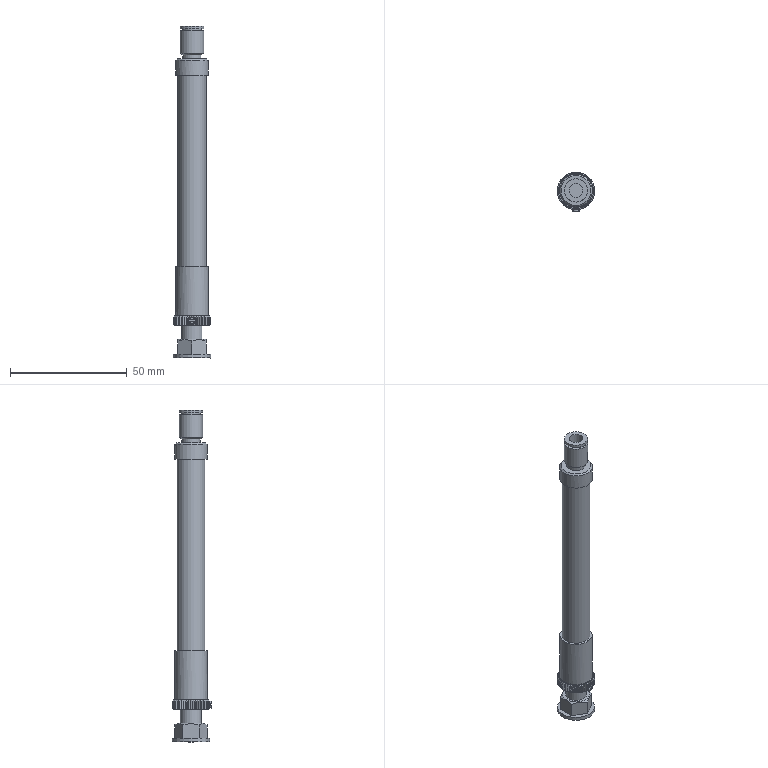Part | NX | features solid 2 | 1 solid | 284 faces | box 16 x 16.9 x 142.1 mm | volume 16500 mm3 | plane 147 | cone 126 | cylinder 11 | commonest cylinder face diameters 8 x2 10 x2 14 x2 3 x1 6 x1 9 x1